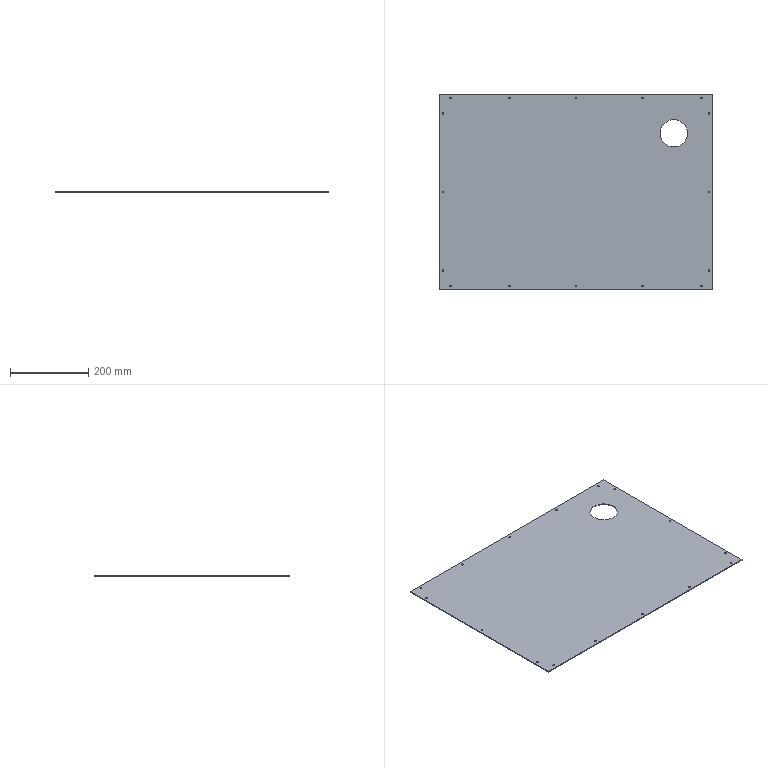Part | SolidWorks | features Extrusion 1, HoleWzd 1, ICE 1 | 1 solid | 40 faces | box 700 x 500 x 2 mm | volume 691794 mm3 | cylinder 34 | plane 6 | commonest cylinder face diameters 4.5 x32 70 x2
STEP:
#1=CARTESIAN_POINT('',(215.,150.,0.));
#2=VERTEX_POINT('',#1);
#3=CARTESIAN_POINT('',(285.,150.,0.));
#4=VERTEX_POINT('',#3);
#5=CARTESIAN_POINT('',(250.,150.,0.));
#6=DIRECTION('',(0.,0.,1.));
#7=DIRECTION('',(1.,0.,0.));
#8=AXIS2_PLACEMENT_3D('',#5,#6,#7);
#9=CIRCLE('',#8,35.);
#10=EDGE_CURVE('',#2,#4,#9,.T.);
#11=ORIENTED_EDGE('',*,*,#10,.F.);
#12=CARTESIAN_POINT('',(215.,150.,2.));
#13=VERTEX_POINT('',#12);
#14=CARTESIAN_POINT('',(215.,150.,-8.));
#15=DIRECTION('',(0.,0.,1.));
#16=VECTOR('',#15,1000.);
#17=LINE('',#14,#16);
#18=EDGE_CURVE('',#2,#13,#17,.T.);
#19=ORIENTED_EDGE('',*,*,#18,.T.);
#20=CARTESIAN_POINT('',(285.,150.,2.));
#21=VERTEX_POINT('',#20);
#22=CARTESIAN_POINT('',(250.,150.,2.));
#23=DIRECTION('',(0.,0.,1.));
#24=DIRECTION('',(1.,0.,0.));
#25=AXIS2_PLACEMENT_3D('',#22,#23,#24);
#26=CIRCLE('',#25,35.);
#27=EDGE_CURVE('',#13,#21,#26,.T.);
#28=ORIENTED_EDGE('',*,*,#27,.T.);
#29=CARTESIAN_POINT('',(285.,150.,-8.));
#30=DIRECTION('',(0.,0.,1.));
#31=VECTOR('',#30,1000.);
#32=LINE('',#29,#31);
#33=EDGE_CURVE('',#4,#21,#32,.T.);
#34=ORIENTED_EDGE('',*,*,#33,.F.);
#35=EDGE_LOOP('',(#11,#19,#28,#34));
#36=FACE_OUTER_BOUND('',#35,.T.);
#37=CARTESIAN_POINT('',(250.,150.,-8.));
#38=DIRECTION('',(0.,0.,1.));
#39=DIRECTION('',(1.,0.,0.));
#40=AXIS2_PLACEMENT_3D('',#37,#38,#39);
#41=CYLINDRICAL_SURFACE('',#40,35.);
#42=ADVANCED_FACE('',(#36),#41,.F.);
#43=CARTESIAN_POINT('',(-342.25,0.,0.));
#44=VERTEX_POINT('',#43);
#45=CARTESIAN_POINT('',(-337.75,0.,0.));
#46=VERTEX_POINT('',#45);
#47=CARTESIAN_POINT('',(-340.,0.,0.));
#48=DIRECTION('',(0.,0.,1.));
#49=DIRECTION('',(1.,0.,0.));
#50=AXIS2_PLACEMENT_3D('',#47,#48,#49);
#51=CIRCLE('',#50,2.25);
#52=EDGE_CURVE('',#44,#46,#51,.T.);
#53=ORIENTED_EDGE('',*,*,#52,.F.);
#54=CARTESIAN_POINT('',(-342.25,0.,2.));
#55=VERTEX_POINT('',#54);
#56=CARTESIAN_POINT('',(-342.25,0.,2.));
#57=DIRECTION('',(0.,0.,1.));
#58=VECTOR('',#57,1000.);
#59=LINE('',#56,#58);
#60=EDGE_CURVE('',#44,#55,#59,.T.);
#61=ORIENTED_EDGE('',*,*,#60,.T.);
#62=CARTESIAN_POINT('',(-337.75,0.,2.));
#63=VERTEX_POINT('',#62);
#64=CARTESIAN_POINT('',(-340.,0.,2.));
#65=DIRECTION('',(0.,0.,1.));
#66=DIRECTION('',(1.,0.,0.));
#67=AXIS2_PLACEMENT_3D('',#64,#65,#66);
#68=CIRCLE('',#67,2.25);
#69=EDGE_CURVE('',#55,#63,#68,.T.);
#70=ORIENTED_EDGE('',*,*,#69,.T.);
#71=CARTESIAN_POINT('',(-337.75,0.,2.));
#72=DIRECTION('',(0.,0.,1.));
#73=VECTOR('',#72,1000.);
#74=LINE('',#71,#73);
#75=EDGE_CURVE('',#46,#63,#74,.T.);
#76=ORIENTED_EDGE('',*,*,#75,.F.);
#77=EDGE_LOOP('',(#53,#61,#70,#76));
#78=FACE_OUTER_BOUND('',#77,.T.);
#79=CARTESIAN_POINT('',(-340.,0.,2.));
#80=DIRECTION('',(0.,0.,1.));
#81=DIRECTION('',(1.,0.,0.));
#82=AXIS2_PLACEMENT_3D('',#79,#80,#81);
#83=CYLINDRICAL_SURFACE('',#82,2.25);
#84=ADVANCED_FACE('',(#78),#83,.F.);
#85=CARTESIAN_POINT('',(-2.25,-240.,0.));
#86=VERTEX_POINT('',#85);
#87=CARTESIAN_POINT('',(2.25,-240.,0.));
#88=VERTEX_POINT('',#87);
#89=CARTESIAN_POINT('',(0.,-240.,0.));
#90=DIRECTION('',(0.,0.,1.));
#91=DIRECTION('',(1.,0.,0.));
#92=AXIS2_PLACEMENT_3D('',#89,#90,#91);
#93=CIRCLE('',#92,2.25);
#94=EDGE_CURVE('',#86,#88,#93,.T.);
#95=ORIENTED_EDGE('',*,*,#94,.F.);
#96=CARTESIAN_POINT('',(-2.25,-240.,2.));
#97=VERTEX_POINT('',#96);
#98=CARTESIAN_POINT('',(-2.25,-240.,2.));
#99=DIRECTION('',(0.,0.,1.));
#100=VECTOR('',#99,1000.);
#101=LINE('',#98,#100);
#102=EDGE_CURVE('',#86,#97,#101,.T.);
#103=ORIENTED_EDGE('',*,*,#102,.T.);
#104=CARTESIAN_POINT('',(2.25,-240.,2.));
#105=VERTEX_POINT('',#104);
#106=CARTESIAN_POINT('',(0.,-240.,2.));
#107=DIRECTION('',(0.,0.,1.));
#108=DIRECTION('',(1.,0.,0.));
#109=AXIS2_PLACEMENT_3D('',#106,#107,#108);
#110=CIRCLE('',#109,2.25);
#111=EDGE_CURVE('',#97,#105,#110,.T.);
#112=ORIENTED_EDGE('',*,*,#111,.T.);
#113=CARTESIAN_POINT('',(2.25,-240.,2.));
#114=DIRECTION('',(0.,0.,1.));
#115=VECTOR('',#114,1000.);
#116=LINE('',#113,#115);
#117=EDGE_CURVE('',#88,#105,#116,.T.);
#118=ORIENTED_EDGE('',*,*,#117,.F.);
#119=EDGE_LOOP('',(#95,#103,#112,#118));
#120=FACE_OUTER_BOUND('',#119,.T.);
#121=CARTESIAN_POINT('',(0.,-240.,2.));
#122=DIRECTION('',(0.,0.,1.));
#123=DIRECTION('',(1.,0.,0.));
#124=AXIS2_PLACEMENT_3D('',#121,#122,#123);
#125=CYLINDRICAL_SURFACE('',#124,2.25);
#126=ADVANCED_FACE('',(#120),#125,.F.);
#127=CARTESIAN_POINT('',(337.75,0.,0.));
#128=VERTEX_POINT('',#127);
#129=CARTESIAN_POINT('',(342.25,0.,0.));
#130=VERTEX_POINT('',#129);
#131=CARTESIAN_POINT('',(340.,0.,0.));
#132=DIRECTION('',(0.,0.,1.));
#133=DIRECTION('',(1.,0.,0.));
#134=AXIS2_PLACEMENT_3D('',#131,#132,#133);
#135=CIRCLE('',#134,2.25);
#136=EDGE_CURVE('',#128,#130,#135,.T.);
#137=ORIENTED_EDGE('',*,*,#136,.F.);
#138=CARTESIAN_POINT('',(337.75,0.,2.));
#139=VERTEX_POINT('',#138);
#140=CARTESIAN_POINT('',(337.75,0.,2.));
#141=DIRECTION('',(0.,0.,1.));
#142=VECTOR('',#141,1000.);
#143=LINE('',#140,#142);
#144=EDGE_CURVE('',#128,#139,#143,.T.);
#145=ORIENTED_EDGE('',*,*,#144,.T.);
#146=CARTESIAN_POINT('',(342.25,0.,2.));
#147=VERTEX_POINT('',#146);
#148=CARTESIAN_POINT('',(340.,0.,2.));
#149=DIRECTION('',(0.,0.,1.));
#150=DIRECTION('',(1.,0.,0.));
#151=AXIS2_PLACEMENT_3D('',#148,#149,#150);
#152=CIRCLE('',#151,2.25);
#153=EDGE_CURVE('',#139,#147,#152,.T.);
#154=ORIENTED_EDGE('',*,*,#153,.T.);
#155=CARTESIAN_POINT('',(342.25,0.,2.));
#156=DIRECTION('',(0.,0.,1.));
#157=VECTOR('',#156,1000.);
#158=LINE('',#155,#157);
#159=EDGE_CURVE('',#130,#147,#158,.T.);
#160=ORIENTED_EDGE('',*,*,#159,.F.);
#161=EDGE_LOOP('',(#137,#145,#154,#160));
#162=FACE_OUTER_BOUND('',#161,.T.);
#163=CARTESIAN_POINT('',(340.,0.,2.));
#164=DIRECTION('',(0.,0.,1.));
#165=DIRECTION('',(1.,0.,0.));
#166=AXIS2_PLACEMENT_3D('',#163,#164,#165);
#167=CYLINDRICAL_SURFACE('',#166,2.25);
#168=ADVANCED_FACE('',(#162),#167,.F.);
#169=CARTESIAN_POINT('',(-2.25,240.,0.));
#170=VERTEX_POINT('',#169);
#171=CARTESIAN_POINT('',(2.25,240.,0.));
#172=VERTEX_POINT('',#171);
#173=CARTESIAN_POINT('',(0.,240.,0.));
#174=DIRECTION('',(0.,0.,1.));
#175=DIRECTION('',(1.,0.,0.));
#176=AXIS2_PLACEMENT_3D('',#173,#174,#175);
#177=CIRCLE('',#176,2.25);
#178=EDGE_CURVE('',#170,#172,#177,.T.);
#179=ORIENTED_EDGE('',*,*,#178,.F.);
#180=CARTESIAN_POINT('',(-2.25,240.,2.));
#181=VERTEX_POINT('',#180);
#182=CARTESIAN_POINT('',(-2.25,240.,2.));
#183=DIRECTION('',(0.,0.,1.));
#184=VECTOR('',#183,1000.);
#185=LINE('',#182,#184);
#186=EDGE_CURVE('',#170,#181,#185,.T.);
#187=ORIENTED_EDGE('',*,*,#186,.T.);
#188=CARTESIAN_POINT('',(2.25,240.,2.));
#189=VERTEX_POINT('',#188);
#190=CARTESIAN_POINT('',(0.,240.,2.));
#191=DIRECTION('',(0.,0.,1.));
#192=DIRECTION('',(1.,0.,0.));
#193=AXIS2_PLACEMENT_3D('',#190,#191,#192);
#194=CIRCLE('',#193,2.25);
#195=EDGE_CURVE('',#181,#189,#194,.T.);
#196=ORIENTED_EDGE('',*,*,#195,.T.);
#197=CARTESIAN_POINT('',(2.25,240.,2.));
#198=DIRECTION('',(0.,0.,1.));
#199=VECTOR('',#198,1000.);
#200=LINE('',#197,#199);
#201=EDGE_CURVE('',#172,#189,#200,.T.);
#202=ORIENTED_EDGE('',*,*,#201,.F.);
#203=EDGE_LOOP('',(#179,#187,#196,#202));
#204=FACE_OUTER_BOUND('',#203,.T.);
#205=CARTESIAN_POINT('',(0.,240.,2.));
#206=DIRECTION('',(0.,0.,1.));
#207=DIRECTION('',(1.,0.,0.));
#208=AXIS2_PLACEMENT_3D('',#205,#206,#207);
#209=CYLINDRICAL_SURFACE('',#208,2.25);
#210=ADVANCED_FACE('',(#204),#209,.F.);
#211=CARTESIAN_POINT('',(-172.25,240.,0.));
#212=VERTEX_POINT('',#211);
#213=CARTESIAN_POINT('',(-167.75,240.,0.));
#214=VERTEX_POINT('',#213);
#215=CARTESIAN_POINT('',(-170.,240.,0.));
#216=DIRECTION('',(0.,0.,1.));
#217=DIRECTION('',(1.,0.,0.));
#218=AXIS2_PLACEMENT_3D('',#215,#216,#217);
#219=CIRCLE('',#218,2.25);
#220=EDGE_CURVE('',#212,#214,#219,.T.);
#221=ORIENTED_EDGE('',*,*,#220,.F.);
#222=CARTESIAN_POINT('',(-172.25,240.,2.));
#223=VERTEX_POINT('',#222);
#224=CARTESIAN_POINT('',(-172.25,240.,2.));
#225=DIRECTION('',(0.,0.,1.));
#226=VECTOR('',#225,1000.);
#227=LINE('',#224,#226);
#228=EDGE_CURVE('',#212,#223,#227,.T.);
#229=ORIENTED_EDGE('',*,*,#228,.T.);
#230=CARTESIAN_POINT('',(-167.75,240.,2.));
#231=VERTEX_POINT('',#230);
#232=CARTESIAN_POINT('',(-170.,240.,2.));
#233=DIRECTION('',(0.,0.,1.));
#234=DIRECTION('',(1.,0.,0.));
#235=AXIS2_PLACEMENT_3D('',#232,#233,#234);
#236=CIRCLE('',#235,2.25);
#237=EDGE_CURVE('',#223,#231,#236,.T.);
#238=ORIENTED_EDGE('',*,*,#237,.T.);
#239=CARTESIAN_POINT('',(-167.75,240.,2.));
#240=DIRECTION('',(0.,0.,1.));
#241=VECTOR('',#240,1000.);
#242=LINE('',#239,#241);
#243=EDGE_CURVE('',#214,#231,#242,.T.);
#244=ORIENTED_EDGE('',*,*,#243,.F.);
#245=EDGE_LOOP('',(#221,#229,#238,#244));
#246=FACE_OUTER_BOUND('',#245,.T.);
#247=CARTESIAN_POINT('',(-170.,240.,2.));
#248=DIRECTION('',(0.,0.,1.));
#249=DIRECTION('',(1.,0.,0.));
#250=AXIS2_PLACEMENT_3D('',#247,#248,#249);
#251=CYLINDRICAL_SURFACE('',#250,2.25);
#252=ADVANCED_FACE('',(#246),#251,.F.);
#253=CARTESIAN_POINT('',(167.75,240.,0.));
#254=VERTEX_POINT('',#253);
#255=CARTESIAN_POINT('',(172.25,240.,0.));
#256=VERTEX_POINT('',#255);
#257=CARTESIAN_POINT('',(170.,240.,0.));
#258=DIRECTION('',(0.,0.,1.));
#259=DIRECTION('',(1.,0.,0.));
#260=AXIS2_PLACEMENT_3D('',#257,#258,#259);
#261=CIRCLE('',#260,2.25);
#262=EDGE_CURVE('',#254,#256,#261,.T.);
#263=ORIENTED_EDGE('',*,*,#262,.F.);
#264=CARTESIAN_POINT('',(167.75,240.,2.));
#265=VERTEX_POINT('',#264);
#266=CARTESIAN_POINT('',(167.75,240.,2.));
#267=DIRECTION('',(0.,0.,1.));
#268=VECTOR('',#267,1000.);
#269=LINE('',#266,#268);
#270=EDGE_CURVE('',#254,#265,#269,.T.);
#271=ORIENTED_EDGE('',*,*,#270,.T.);
#272=CARTESIAN_POINT('',(172.25,240.,2.));
#273=VERTEX_POINT('',#272);
#274=CARTESIAN_POINT('',(170.,240.,2.));
#275=DIRECTION('',(0.,0.,1.));
#276=DIRECTION('',(1.,0.,0.));
#277=AXIS2_PLACEMENT_3D('',#274,#275,#276);
#278=CIRCLE('',#277,2.25);
#279=EDGE_CURVE('',#265,#273,#278,.T.);
#280=ORIENTED_EDGE('',*,*,#279,.T.);
#281=CARTESIAN_POINT('',(172.25,240.,2.));
#282=DIRECTION('',(0.,0.,1.));
#283=VECTOR('',#282,1000.);
#284=LINE('',#281,#283);
#285=EDGE_CURVE('',#256,#273,#284,.T.);
#286=ORIENTED_EDGE('',*,*,#285,.F.);
#287=EDGE_LOOP('',(#263,#271,#280,#286));
#288=FACE_OUTER_BOUND('',#287,.T.);
#289=CARTESIAN_POINT('',(170.,240.,2.));
#290=DIRECTION('',(0.,0.,1.));
#291=DIRECTION('',(1.,0.,0.));
#292=AXIS2_PLACEMENT_3D('',#289,#290,#291);
#293=CYLINDRICAL_SURFACE('',#292,2.25);
#294=ADVANCED_FACE('',(#288),#293,.F.);
#295=CARTESIAN_POINT('',(-172.25,-240.,0.));
#296=VERTEX_POINT('',#295);
#297=CARTESIAN_POINT('',(-167.75,-240.,0.));
#298=VERTEX_POINT('',#297);
#299=CARTESIAN_POINT('',(-170.,-240.,0.));
#300=DIRECTION('',(0.,0.,1.));
#301=DIRECTION('',(1.,0.,0.));
#302=AXIS2_PLACEMENT_3D('',#299,#300,#301);
#303=CIRCLE('',#302,2.25);
#304=EDGE_CURVE('',#296,#298,#303,.T.);
#305=ORIENTED_EDGE('',*,*,#304,.F.);
#306=CARTESIAN_POINT('',(-172.25,-240.,2.));
#307=VERTEX_POINT('',#306);
#308=CARTESIAN_POINT('',(-172.25,-240.,2.));
#309=DIRECTION('',(0.,0.,1.));
#310=VECTOR('',#309,1000.);
#311=LINE('',#308,#310);
#312=EDGE_CURVE('',#296,#307,#311,.T.);
#313=ORIENTED_EDGE('',*,*,#312,.T.);
#314=CARTESIAN_POINT('',(-167.75,-240.,2.));
#315=VERTEX_POINT('',#314);
#316=CARTESIAN_POINT('',(-170.,-240.,2.));
#317=DIRECTION('',(0.,0.,1.));
#318=DIRECTION('',(1.,0.,0.));
#319=AXIS2_PLACEMENT_3D('',#316,#317,#318);
#320=CIRCLE('',#319,2.25);
#321=EDGE_CURVE('',#307,#315,#320,.T.);
#322=ORIENTED_EDGE('',*,*,#321,.T.);
#323=CARTESIAN_POINT('',(-167.75,-240.,2.));
#324=DIRECTION('',(0.,0.,1.));
#325=VECTOR('',#324,1000.);
#326=LINE('',#323,#325);
#327=EDGE_CURVE('',#298,#315,#326,.T.);
#328=ORIENTED_EDGE('',*,*,#327,.F.);
#329=EDGE_LOOP('',(#305,#313,#322,#328));
#330=FACE_OUTER_BOUND('',#329,.T.);
#331=CARTESIAN_POINT('',(-170.,-240.,2.));
#332=DIRECTION('',(0.,0.,1.));
#333=DIRECTION('',(1.,0.,0.));
#334=AXIS2_PLACEMENT_3D('',#331,#332,#333);
#335=CYLINDRICAL_SURFACE('',#334,2.25);
#336=ADVANCED_FACE('',(#330),#335,.F.);
#337=CARTESIAN_POINT('',(167.75,-240.,0.));
#338=VERTEX_POINT('',#337);
#339=CARTESIAN_POINT('',(172.25,-240.,0.));
#340=VERTEX_POINT('',#339);
#341=CARTESIAN_POINT('',(170.,-240.,0.));
#342=DIRECTION('',(0.,0.,1.));
#343=DIRECTION('',(1.,0.,0.));
#344=AXIS2_PLACEMENT_3D('',#341,#342,#343);
#345=CIRCLE('',#344,2.25);
#346=EDGE_CURVE('',#338,#340,#345,.T.);
#347=ORIENTED_EDGE('',*,*,#346,.F.);
#348=CARTESIAN_POINT('',(167.75,-240.,2.));
#349=VERTEX_POINT('',#348);
#350=CARTESIAN_POINT('',(167.75,-240.,2.));
#351=DIRECTION('',(0.,0.,1.));
#352=VECTOR('',#351,1000.);
#353=LINE('',#350,#352);
#354=EDGE_CURVE('',#338,#349,#353,.T.);
#355=ORIENTED_EDGE('',*,*,#354,.T.);
#356=CARTESIAN_POINT('',(172.25,-240.,2.));
#357=VERTEX_POINT('',#356);
#358=CARTESIAN_POINT('',(170.,-240.,2.));
#359=DIRECTION('',(0.,0.,1.));
#360=DIRECTION('',(1.,0.,0.));
#361=AXIS2_PLACEMENT_3D('',#358,#359,#360);
#362=CIRCLE('',#361,2.25);
#363=EDGE_CURVE('',#349,#357,#362,.T.);
#364=ORIENTED_EDGE('',*,*,#363,.T.);
#365=CARTESIAN_POINT('',(172.25,-240.,2.));
#366=DIRECTION('',(0.,0.,1.));
#367=VECTOR('',#366,1000.);
#368=LINE('',#365,#367);
#369=EDGE_CURVE('',#340,#357,#368,.T.);
#370=ORIENTED_EDGE('',*,*,#369,.F.);
#371=EDGE_LOOP('',(#347,#355,#364,#370));
#372=FACE_OUTER_BOUND('',#371,.T.);
#373=CARTESIAN_POINT('',(170.,-240.,2.));
#374=DIRECTION('',(0.,0.,1.));
#375=DIRECTION('',(1.,0.,0.));
#376=AXIS2_PLACEMENT_3D('',#373,#374,#375);
#377=CYLINDRICAL_SURFACE('',#376,2.25);
#378=ADVANCED_FACE('',(#372),#377,.F.);
#379=CARTESIAN_POINT('',(-322.25,240.,0.));
#380=VERTEX_POINT('',#379);
#381=CARTESIAN_POINT('',(-317.75,240.,0.));
#382=VERTEX_POINT('',#381);
#383=CARTESIAN_POINT('',(-320.,240.,0.));
#384=DIRECTION('',(0.,0.,1.));
#385=DIRECTION('',(1.,0.,0.));
#386=AXIS2_PLACEMENT_3D('',#383,#384,#385);
#387=CIRCLE('',#386,2.25);
#388=EDGE_CURVE('',#380,#382,#387,.T.);
#389=ORIENTED_EDGE('',*,*,#388,.F.);
#390=CARTESIAN_POINT('',(-322.25,240.,2.));
#391=VERTEX_POINT('',#390);
#392=CARTESIAN_POINT('',(-322.25,240.,2.));
#393=DIRECTION('',(0.,0.,1.));
#394=VECTOR('',#393,1000.);
#395=LINE('',#392,#394);
#396=EDGE_CURVE('',#380,#391,#395,.T.);
#397=ORIENTED_EDGE('',*,*,#396,.T.);
#398=CARTESIAN_POINT('',(-317.75,240.,2.));
#399=VERTEX_POINT('',#398);
#400=CARTESIAN_POINT('',(-320.,240.,2.));
#401=DIRECTION('',(0.,0.,1.));
#402=DIRECTION('',(1.,0.,0.));
#403=AXIS2_PLACEMENT_3D('',#400,#401,#402);
#404=CIRCLE('',#403,2.25);
#405=EDGE_CURVE('',#391,#399,#404,.T.);
#406=ORIENTED_EDGE('',*,*,#405,.T.);
#407=CARTESIAN_POINT('',(-317.75,240.,2.));
#408=DIRECTION('',(0.,0.,1.));
#409=VECTOR('',#408,1000.);
#410=LINE('',#407,#409);
#411=EDGE_CURVE('',#382,#399,#410,.T.);
#412=ORIENTED_EDGE('',*,*,#411,.F.);
#413=EDGE_LOOP('',(#389,#397,#406,#412));
#414=FACE_OUTER_BOUND('',#413,.T.);
#415=CARTESIAN_POINT('',(-320.,240.,2.));
#416=DIRECTION('',(0.,0.,1.));
#417=DIRECTION('',(1.,0.,0.));
#418=AXIS2_PLACEMENT_3D('',#415,#416,#417);
#419=CYLINDRICAL_SURFACE('',#418,2.25);
#420=ADVANCED_FACE('',(#414),#419,.F.);
#421=CARTESIAN_POINT('',(317.75,240.,0.));
#422=VERTEX_POINT('',#421);
#423=CARTESIAN_POINT('',(322.25,240.,0.));
#424=VERTEX_POINT('',#423);
#425=CARTESIAN_POINT('',(320.,240.,0.));
#426=DIRECTION('',(0.,0.,1.));
#427=DIRECTION('',(1.,0.,0.));
#428=AXIS2_PLACEMENT_3D('',#425,#426,#427);
#429=CIRCLE('',#428,2.25);
#430=EDGE_CURVE('',#422,#424,#429,.T.);
#431=ORIENTED_EDGE('',*,*,#430,.F.);
#432=CARTESIAN_POINT('',(317.75,240.,2.));
#433=VERTEX_POINT('',#432);
#434=CARTESIAN_POINT('',(317.75,240.,2.));
#435=DIRECTION('',(0.,0.,1.));
#436=VECTOR('',#435,1000.);
#437=LINE('',#434,#436);
#438=EDGE_CURVE('',#422,#433,#437,.T.);
#439=ORIENTED_EDGE('',*,*,#438,.T.);
#440=CARTESIAN_POINT('',(322.25,240.,2.));
#441=VERTEX_POINT('',#440);
#442=CARTESIAN_POINT('',(320.,240.,2.));
#443=DIRECTION('',(0.,0.,1.));
#444=DIRECTION('',(1.,0.,0.));
#445=AXIS2_PLACEMENT_3D('',#442,#443,#444);
#446=CIRCLE('',#445,2.25);
#447=EDGE_CURVE('',#433,#441,#446,.T.);
#448=ORIENTED_EDGE('',*,*,#447,.T.);
#449=CARTESIAN_POINT('',(322.25,240.,2.));
#450=DIRECTION('',(0.,0.,1.));
#451=VECTOR('',#450,1000.);
#452=LINE('',#449,#451);
#453=EDGE_CURVE('',#424,#441,#452,.T.);
#454=ORIENTED_EDGE('',*,*,#453,.F.);
#455=EDGE_LOOP('',(#431,#439,#448,#454));
#456=FACE_OUTER_BOUND('',#455,.T.);
#457=CARTESIAN_POINT('',(320.,240.,2.));
#458=DIRECTION('',(0.,0.,1.));
#459=DIRECTION('',(1.,0.,0.));
#460=AXIS2_PLACEMENT_3D('',#457,#458,#459);
#461=CYLINDRICAL_SURFACE('',#460,2.25);
#462=ADVANCED_FACE('',(#456),#461,.F.);
#463=CARTESIAN_POINT('',(-342.25,200.,0.));
#464=VERTEX_POINT('',#463);
#465=CARTESIAN_POINT('',(-337.75,200.,0.));
#466=VERTEX_POINT('',#465);
#467=CARTESIAN_POINT('',(-340.,200.,0.));
#468=DIRECTION('',(0.,0.,1.));
#469=DIRECTION('',(1.,0.,0.));
#470=AXIS2_PLACEMENT_3D('',#467,#468,#469);
#471=CIRCLE('',#470,2.25);
#472=EDGE_CURVE('',#464,#466,#471,.T.);
#473=ORIENTED_EDGE('',*,*,#472,.F.);
#474=CARTESIAN_POINT('',(-342.25,200.,2.));
#475=VERTEX_POINT('',#474);
#476=CARTESIAN_POINT('',(-342.25,200.,2.));
#477=DIRECTION('',(0.,0.,1.));
#478=VECTOR('',#477,1000.);
#479=LINE('',#476,#478);
#480=EDGE_CURVE('',#464,#475,#479,.T.);
#481=ORIENTED_EDGE('',*,*,#480,.T.);
#482=CARTESIAN_POINT('',(-337.75,200.,2.));
#483=VERTEX_POINT('',#482);
#484=CARTESIAN_POINT('',(-340.,200.,2.));
#485=DIRECTION('',(0.,0.,1.));
#486=DIRECTION('',(1.,0.,0.));
#487=AXIS2_PLACEMENT_3D('',#484,#485,#486);
#488=CIRCLE('',#487,2.25);
#489=EDGE_CURVE('',#475,#483,#488,.T.);
#490=ORIENTED_EDGE('',*,*,#489,.T.);
#491=CARTESIAN_POINT('',(-337.75,200.,2.));
#492=DIRECTION('',(0.,0.,1.));
#493=VECTOR('',#492,1000.);
#494=LINE('',#491,#493);
#495=EDGE_CURVE('',#466,#483,#494,.T.);
#496=ORIENTED_EDGE('',*,*,#495,.F.);
#497=EDGE_LOOP('',(#473,#481,#490,#496));
#498=FACE_OUTER_BOUND('',#497,.T.);
#499=CARTESIAN_POINT('',(-340.,200.,2.));
#500=DIRECTION('',(0.,0.,1.));
#501=DIRECTION('',(1.,0.,0.));
#502=AXIS2_PLACEMENT_3D('',#499,#500,#501);
#503=CYLINDRICAL_SURFACE('',#502,2.25);
#504=ADVANCED_FACE('',(#498),#503,.F.);
#505=CARTESIAN_POINT('',(-342.25,-200.,0.));
#506=VERTEX_POINT('',#505);
#507=CARTESIAN_POINT('',(-337.75,-200.,0.));
#508=VERTEX_POINT('',#507);
#509=CARTESIAN_POINT('',(-340.,-200.,0.));
#510=DIRECTION('',(0.,0.,1.));
#511=DIRECTION('',(1.,0.,0.));
#512=AXIS2_PLACEMENT_3D('',#509,#510,#511);
#513=CIRCLE('',#512,2.25);
#514=EDGE_CURVE('',#506,#508,#513,.T.);
#515=ORIENTED_EDGE('',*,*,#514,.F.);
#516=CARTESIAN_POINT('',(-342.25,-200.,2.));
#517=VERTEX_POINT('',#516);
#518=CARTESIAN_POINT('',(-342.25,-200.,2.));
#519=DIRECTION('',(0.,0.,1.));
#520=VECTOR('',#519,1000.);
#521=LINE('',#518,#520);
#522=EDGE_CURVE('',#506,#517,#521,.T.);
#523=ORIENTED_EDGE('',*,*,#522,.T.);
#524=CARTESIAN_POINT('',(-337.75,-200.,2.));
#525=VERTEX_POINT('',#524);
#526=CARTESIAN_POINT('',(-340.,-200.,2.));
#527=DIRECTION('',(0.,0.,1.));
#528=DIRECTION('',(1.,0.,0.));
#529=AXIS2_PLACEMENT_3D('',#526,#527,#528);
#530=CIRCLE('',#529,2.25);
#531=EDGE_CURVE('',#517,#525,#530,.T.);
#532=ORIENTED_EDGE('',*,*,#531,.T.);
#533=CARTESIAN_POINT('',(-337.75,-200.,2.));
#534=DIRECTION('',(0.,0.,1.));
#535=VECTOR('',#534,1000.);
#536=LINE('',#533,#535);
#537=EDGE_CURVE('',#508,#525,#536,.T.);
#538=ORIENTED_EDGE('',*,*,#537,.F.);
#539=EDGE_LOOP('',(#515,#523,#532,#538));
#540=FACE_OUTER_BOUND('',#539,.T.);
#541=CARTESIAN_POINT('',(-340.,-200.,2.));
#542=DIRECTION('',(0.,0.,1.));
#543=DIRECTION('',(1.,0.,0.));
#544=AXIS2_PLACEMENT_3D('',#541,#542,#543);
#545=CYLINDRICAL_SURFACE('',#544,2.25);
#546=ADVANCED_FACE('',(#540),#545,.F.);
#547=CARTESIAN_POINT('',(337.75,-200.,0.));
#548=VERTEX_POINT('',#547);
#549=CARTESIAN_POINT('',(342.25,-200.,0.));
#550=VERTEX_POINT('',#549);
#551=CARTESIAN_POINT('',(340.,-200.,0.));
#552=DIRECTION('',(0.,0.,1.));
#553=DIRECTION('',(1.,0.,0.));
#554=AXIS2_PLACEMENT_3D('',#551,#552,#553);
#555=CIRCLE('',#554,2.25);
#556=EDGE_CURVE('',#548,#550,#555,.T.);
#557=ORIENTED_EDGE('',*,*,#556,.F.);
#558=CARTESIAN_POINT('',(337.75,-200.,2.));
#559=VERTEX_POINT('',#558);
#560=CARTESIAN_POINT('',(337.75,-200.,2.));
#561=DIRECTION('',(0.,0.,1.));
#562=VECTOR('',#561,1000.);
#563=LINE('',#560,#562);
#564=EDGE_CURVE('',#548,#559,#563,.T.);
#565=ORIENTED_EDGE('',*,*,#564,.T.);
#566=CARTESIAN_POINT('',(342.25,-200.,2.));
#567=VERTEX_POINT('',#566);
#568=CARTESIAN_POINT('',(340.,-200.,2.));
#569=DIRECTION('',(0.,0.,1.));
#570=DIRECTION('',(1.,0.,0.));
#571=AXIS2_PLACEMENT_3D('',#568,#569,#570);
#572=CIRCLE('',#571,2.25);
#573=EDGE_CURVE('',#559,#567,#572,.T.);
#574=ORIENTED_EDGE('',*,*,#573,.T.);
#575=CARTESIAN_POINT('',(342.25,-200.,2.));
#576=DIRECTION('',(0.,0.,1.));
#577=VECTOR('',#576,1000.);
#578=LINE('',#575,#577);
#579=EDGE_CURVE('',#550,#567,#578,.T.);
#580=ORIENTED_EDGE('',*,*,#579,.F.);
#581=EDGE_LOOP('',(#557,#565,#574,#580));
#582=FACE_OUTER_BOUND('',#581,.T.);
#583=CARTESIAN_POINT('',(340.,-200.,2.));
#584=DIRECTION('',(0.,0.,1.));
#585=DIRECTION('',(1.,0.,0.));
#586=AXIS2_PLACEMENT_3D('',#583,#584,#585);
#587=CYLINDRICAL_SURFACE('',#586,2.25);
#588=ADVANCED_FACE('',(#582),#587,.F.);
#589=CARTESIAN_POINT('',(337.75,200.,0.));
#590=VERTEX_POINT('',#589);
#591=CARTESIAN_POINT('',(342.25,200.,0.));
#592=VERTEX_POINT('',#591);
#593=CARTESIAN_POINT('',(340.,200.,0.));
#594=DIRECTION('',(0.,0.,1.));
#595=DIRECTION('',(1.,0.,0.));
#596=AXIS2_PLACEMENT_3D('',#593,#594,#595);
#597=CIRCLE('',#596,2.25);
#598=EDGE_CURVE('',#590,#592,#597,.T.);
#599=ORIENTED_EDGE('',*,*,#598,.F.);
#600=CARTESIAN_POINT('',(337.75,200.,2.));
#601=VERTEX_POINT('',#600);
#602=CARTESIAN_POINT('',(337.75,200.,2.));
#603=DIRECTION('',(0.,0.,1.));
#604=VECTOR('',#603,1000.);
#605=LINE('',#602,#604);
#606=EDGE_CURVE('',#590,#601,#605,.T.);
#607=ORIENTED_EDGE('',*,*,#606,.T.);
#608=CARTESIAN_POINT('',(342.25,200.,2.));
#609=VERTEX_POINT('',#608);
#610=CARTESIAN_POINT('',(340.,200.,2.));
#611=DIRECTION('',(0.,0.,1.));
#612=DIRECTION('',(1.,0.,0.));
#613=AXIS2_PLACEMENT_3D('',#610,#611,#612);
#614=CIRCLE('',#613,2.25);
#615=EDGE_CURVE('',#601,#609,#614,.T.);
#616=ORIENTED_EDGE('',*,*,#615,.T.);
#617=CARTESIAN_POINT('',(342.25,200.,2.));
#618=DIRECTION('',(0.,0.,1.));
#619=VECTOR('',#618,1000.);
#620=LINE('',#617,#619);
#621=EDGE_CURVE('',#592,#609,#620,.T.);
#622=ORIENTED_EDGE('',*,*,#621,.F.);
#623=EDGE_LOOP('',(#599,#607,#616,#622));
#624=FACE_OUTER_BOUND('',#623,.T.);
#625=CARTESIAN_POINT('',(340.,200.,2.));
#626=DIRECTION('',(0.,0.,1.));
#627=DIRECTION('',(1.,0.,0.));
#628=AXIS2_PLACEMENT_3D('',#625,#626,#627);
#629=CYLINDRICAL_SURFACE('',#628,2.25);
#630=ADVANCED_FACE('',(#624),#629,.F.);
#631=CARTESIAN_POINT('',(-322.25,-240.,0.));
#632=VERTEX_POINT('',#631);
#633=CARTESIAN_POINT('',(-317.75,-240.,0.));
#634=VERTEX_POINT('',#633);
#635=CARTESIAN_POINT('',(-320.,-240.,0.));
#636=DIRECTION('',(0.,0.,1.));
#637=DIRECTION('',(1.,0.,0.));
#638=AXIS2_PLACEMENT_3D('',#635,#636,#637);
#639=CIRCLE('',#638,2.25);
#640=EDGE_CURVE('',#632,#634,#639,.T.);
#641=ORIENTED_EDGE('',*,*,#640,.F.);
#642=CARTESIAN_POINT('',(-322.25,-240.,2.));
#643=VERTEX_POINT('',#642);
#644=CARTESIAN_POINT('',(-322.25,-240.,2.));
#645=DIRECTION('',(0.,0.,1.));
#646=VECTOR('',#645,1000.);
#647=LINE('',#644,#646);
#648=EDGE_CURVE('',#632,#643,#647,.T.);
#649=ORIENTED_EDGE('',*,*,#648,.T.);
#650=CARTESIAN_POINT('',(-317.75,-240.,2.));
#651=VERTEX_POINT('',#650);
#652=CARTESIAN_POINT('',(-320.,-240.,2.));
#653=DIRECTION('',(0.,0.,1.));
#654=DIRECTION('',(1.,0.,0.));
#655=AXIS2_PLACEMENT_3D('',#652,#653,#654);
#656=CIRCLE('',#655,2.25);
#657=EDGE_CURVE('',#643,#651,#656,.T.);
#658=ORIENTED_EDGE('',*,*,#657,.T.);
#659=CARTESIAN_POINT('',(-317.75,-240.,2.));
#660=DIRECTION('',(0.,0.,1.));
#661=VECTOR('',#660,1000.);
#662=LINE('',#659,#661);
#663=EDGE_CURVE('',#634,#651,#662,.T.);
#664=ORIENTED_EDGE('',*,*,#663,.F.);
#665=EDGE_LOOP('',(#641,#649,#658,#664));
#666=FACE_OUTER_BOUND('',#665,.T.);
#667=CARTESIAN_POINT('',(-320.,-240.,2.));
#668=DIRECTION('',(0.,0.,1.));
#669=DIRECTION('',(1.,0.,0.));
#670=AXIS2_PLACEMENT_3D('',#667,#668,#669);
#671=CYLINDRICAL_SURFACE('',#670,2.25);
#672=ADVANCED_FACE('',(#666),#671,.F.);
#673=CARTESIAN_POINT('',(317.75,-240.,0.));
#674=VERTEX_POINT('',#673);
#675=CARTESIAN_POINT('',(322.25,-240.,0.));
#676=VERTEX_POINT('',#675);
#677=CARTESIAN_POINT('',(320.,-240.,0.));
#678=DIRECTION('',(0.,0.,1.));
#679=DIRECTION('',(1.,0.,0.));
#680=AXIS2_PLACEMENT_3D('',#677,#678,#679);
#681=CIRCLE('',#680,2.25);
#682=EDGE_CURVE('',#674,#676,#681,.T.);
#683=ORIENTED_EDGE('',*,*,#682,.F.);
#684=CARTESIAN_POINT('',(317.75,-240.,2.));
#685=VERTEX_POINT('',#684);
#686=CARTESIAN_POINT('',(317.75,-240.,2.));
#687=DIRECTION('',(0.,0.,1.));
#688=VECTOR('',#687,1000.);
#689=LINE('',#686,#688);
#690=EDGE_CURVE('',#674,#685,#689,.T.);
#691=ORIENTED_EDGE('',*,*,#690,.T.);
#692=CARTESIAN_POINT('',(322.25,-240.,2.));
#693=VERTEX_POINT('',#692);
#694=CARTESIAN_POINT('',(320.,-240.,2.));
#695=DIRECTION('',(0.,0.,1.));
#696=DIRECTION('',(1.,0.,0.));
#697=AXIS2_PLACEMENT_3D('',#694,#695,#696);
#698=CIRCLE('',#697,2.25);
#699=EDGE_CURVE('',#685,#693,#698,.T.);
#700=ORIENTED_EDGE('',*,*,#699,.T.);
#701=CARTESIAN_POINT('',(322.25,-240.,2.));
#702=DIRECTION('',(0.,0.,1.));
#703=VECTOR('',#702,1000.);
#704=LINE('',#701,#703);
#705=EDGE_CURVE('',#676,#693,#704,.T.);
#706=ORIENTED_EDGE('',*,*,#705,.F.);
#707=EDGE_LOOP('',(#683,#691,#700,#706));
#708=FACE_OUTER_BOUND('',#707,.T.);
#709=CARTESIAN_POINT('',(320.,-240.,2.));
#710=DIRECTION('',(0.,0.,1.));
#711=DIRECTION('',(1.,0.,0.));
#712=AXIS2_PLACEMENT_3D('',#709,#710,#711);
#713=CYLINDRICAL_SURFACE('',#712,2.25);
#714=ADVANCED_FACE('',(#708),#713,.F.);
#715=CARTESIAN_POINT('',(350.,-250.,0.));
#716=VERTEX_POINT('',#715);
#717=CARTESIAN_POINT('',(350.,250.,0.));
#718=VERTEX_POINT('',#717);
#719=CARTESIAN_POINT('',(350.,250.,0.));
#720=DIRECTION('',(0.,1.,0.));
#721=VECTOR('',#720,1000.);
#722=LINE('',#719,#721);
#723=EDGE_CURVE('',#716,#718,#722,.T.);
#724=ORIENTED_EDGE('',*,*,#723,.T.);
#725=CARTESIAN_POINT('',(350.,250.,2.));
#726=VERTEX_POINT('',#725);
#727=CARTESIAN_POINT('',(350.,250.,2.));
#728=DIRECTION('',(0.,0.,-1.));
#729=VECTOR('',#728,1000.);
#730=LINE('',#727,#729);
#731=EDGE_CURVE('',#726,#718,#730,.T.);
#732=ORIENTED_EDGE('',*,*,#731,.F.);
#733=CARTESIAN_POINT('',(350.,-250.,2.));
#734=VERTEX_POINT('',#733);
#735=CARTESIAN_POINT('',(350.,250.,2.));
#736=DIRECTION('',(0.,1.,0.));
#737=VECTOR('',#736,1000.);
#738=LINE('',#735,#737);
#739=EDGE_CURVE('',#734,#726,#738,.T.);
#740=ORIENTED_EDGE('',*,*,#739,.F.);
#741=CARTESIAN_POINT('',(350.,-250.,2.));
#742=DIRECTION('',(0.,0.,-1.));
#743=VECTOR('',#742,1000.);
#744=LINE('',#741,#743);
#745=EDGE_CURVE('',#734,#716,#744,.T.);
#746=ORIENTED_EDGE('',*,*,#745,.T.);
#747=EDGE_LOOP('',(#724,#732,#740,#746));
#748=FACE_OUTER_BOUND('',#747,.T.);
#749=CARTESIAN_POINT('',(350.,250.,2.));
#750=DIRECTION('',(-1.,0.,0.));
#751=DIRECTION('',(0.,0.,1.));
#752=AXIS2_PLACEMENT_3D('',#749,#750,#751);
#753=PLANE('',#752);
#754=ADVANCED_FACE('',(#748),#753,.F.);
#755=CARTESIAN_POINT('',(-350.,250.,0.));
#756=VERTEX_POINT('',#755);
#757=CARTESIAN_POINT('',(-350.,250.,0.));
#758=DIRECTION('',(-1.,0.,0.));
#759=VECTOR('',#758,1000.);
#760=LINE('',#757,#759);
#761=EDGE_CURVE('',#718,#756,#760,.T.);
#762=ORIENTED_EDGE('',*,*,#761,.T.);
#763=CARTESIAN_POINT('',(-350.,250.,2.));
#764=VERTEX_POINT('',#763);
#765=CARTESIAN_POINT('',(-350.,250.,2.));
#766=DIRECTION('',(0.,0.,-1.));
#767=VECTOR('',#766,1000.);
#768=LINE('',#765,#767);
#769=EDGE_CURVE('',#764,#756,#768,.T.);
#770=ORIENTED_EDGE('',*,*,#769,.F.);
#771=CARTESIAN_POINT('',(-350.,250.,2.));
#772=DIRECTION('',(-1.,0.,0.));
#773=VECTOR('',#772,1000.);
#774=LINE('',#771,#773);
#775=EDGE_CURVE('',#726,#764,#774,.T.);
#776=ORIENTED_EDGE('',*,*,#775,.F.);
#777=ORIENTED_EDGE('',*,*,#731,.T.);
#778=EDGE_LOOP('',(#762,#770,#776,#777));
#779=FACE_OUTER_BOUND('',#778,.T.);
#780=CARTESIAN_POINT('',(-350.,250.,2.));
#781=DIRECTION('',(0.,-1.,0.));
#782=DIRECTION('',(0.,0.,-1.));
#783=AXIS2_PLACEMENT_3D('',#780,#781,#782);
#784=PLANE('',#783);
#785=ADVANCED_FACE('',(#779),#784,.F.);
#786=CARTESIAN_POINT('',(-350.,-250.,0.));
#787=VERTEX_POINT('',#786);
#788=CARTESIAN_POINT('',(-350.,250.,0.));
#789=DIRECTION('',(0.,-1.,0.));
#790=VECTOR('',#789,1000.);
#791=LINE('',#788,#790);
#792=EDGE_CURVE('',#756,#787,#791,.T.);
#793=ORIENTED_EDGE('',*,*,#792,.T.);
#794=CARTESIAN_POINT('',(-350.,-250.,2.));
#795=VERTEX_POINT('',#794);
#796=CARTESIAN_POINT('',(-350.,-250.,2.));
#797=DIRECTION('',(0.,0.,-1.));
#798=VECTOR('',#797,1000.);
#799=LINE('',#796,#798);
#800=EDGE_CURVE('',#795,#787,#799,.T.);
#801=ORIENTED_EDGE('',*,*,#800,.F.);
#802=CARTESIAN_POINT('',(-350.,250.,2.));
#803=DIRECTION('',(0.,-1.,0.));
#804=VECTOR('',#803,1000.);
#805=LINE('',#802,#804);
#806=EDGE_CURVE('',#764,#795,#805,.T.);
#807=ORIENTED_EDGE('',*,*,#806,.F.);
#808=ORIENTED_EDGE('',*,*,#769,.T.);
#809=EDGE_LOOP('',(#793,#801,#807,#808));
#810=FACE_OUTER_BOUND('',#809,.T.);
#811=CARTESIAN_POINT('',(-350.,250.,2.));
#812=DIRECTION('',(1.,0.,0.));
#813=DIRECTION('',(0.,0.,-1.));
#814=AXIS2_PLACEMENT_3D('',#811,#812,#813);
#815=PLANE('',#814);
#816=ADVANCED_FACE('',(#810),#815,.F.);
#817=CARTESIAN_POINT('',(-350.,-250.,0.));
#818=DIRECTION('',(1.,0.,0.));
#819=VECTOR('',#818,1000.);
#820=LINE('',#817,#819);
#821=EDGE_CURVE('',#787,#716,#820,.T.);
#822=ORIENTED_EDGE('',*,*,#821,.T.);
#823=ORIENTED_EDGE('',*,*,#745,.F.);
#824=CARTESIAN_POINT('',(-350.,-250.,2.));
#825=DIRECTION('',(1.,0.,0.));
#826=VECTOR('',#825,1000.);
#827=LINE('',#824,#826);
#828=EDGE_CURVE('',#795,#734,#827,.T.);
#829=ORIENTED_EDGE('',*,*,#828,.F.);
#830=ORIENTED_EDGE('',*,*,#800,.T.);
#831=EDGE_LOOP('',(#822,#823,#829,#830));
#832=FACE_OUTER_BOUND('',#831,.T.);
#833=CARTESIAN_POINT('',(-350.,-250.,2.));
#834=DIRECTION('',(0.,1.,0.));
#835=DIRECTION('',(0.,0.,1.));
#836=AXIS2_PLACEMENT_3D('',#833,#834,#835);
#837=PLANE('',#836);
#838=ADVANCED_FACE('',(#832),#837,.F.);
#839=CARTESIAN_POINT('',(250.,150.,2.));
#840=DIRECTION('',(0.,0.,1.));
#841=DIRECTION('',(1.,0.,0.));
#842=AXIS2_PLACEMENT_3D('',#839,#840,#841);
#843=CIRCLE('',#842,35.);
#844=EDGE_CURVE('',#21,#13,#843,.T.);
#845=ORIENTED_EDGE('',*,*,#844,.F.);
#846=ORIENTED_EDGE('',*,*,#27,.F.);
#847=EDGE_LOOP('',(#845,#846));
#848=FACE_BOUND('',#847,.T.);
#849=CARTESIAN_POINT('',(-340.,0.,2.));
#850=DIRECTION('',(0.,0.,1.));
#851=DIRECTION('',(1.,0.,0.));
#852=AXIS2_PLACEMENT_3D('',#849,#850,#851);
#853=CIRCLE('',#852,2.25);
#854=EDGE_CURVE('',#63,#55,#853,.T.);
#855=ORIENTED_EDGE('',*,*,#854,.F.);
#856=ORIENTED_EDGE('',*,*,#69,.F.);
#857=EDGE_LOOP('',(#855,#856));
#858=FACE_BOUND('',#857,.T.);
#859=CARTESIAN_POINT('',(0.,-240.,2.));
#860=DIRECTION('',(0.,0.,1.));
#861=DIRECTION('',(1.,0.,0.));
#862=AXIS2_PLACEMENT_3D('',#859,#860,#861);
#863=CIRCLE('',#862,2.25);
#864=EDGE_CURVE('',#105,#97,#863,.T.);
#865=ORIENTED_EDGE('',*,*,#864,.F.);
#866=ORIENTED_EDGE('',*,*,#111,.F.);
#867=EDGE_LOOP('',(#865,#866));
#868=FACE_BOUND('',#867,.T.);
#869=CARTESIAN_POINT('',(340.,0.,2.));
#870=DIRECTION('',(0.,0.,1.));
#871=DIRECTION('',(1.,0.,0.));
#872=AXIS2_PLACEMENT_3D('',#869,#870,#871);
#873=CIRCLE('',#872,2.25);
#874=EDGE_CURVE('',#147,#139,#873,.T.);
#875=ORIENTED_EDGE('',*,*,#874,.F.);
#876=ORIENTED_EDGE('',*,*,#153,.F.);
#877=EDGE_LOOP('',(#875,#876));
#878=FACE_BOUND('',#877,.T.);
#879=CARTESIAN_POINT('',(0.,240.,2.));
#880=DIRECTION('',(0.,0.,1.));
#881=DIRECTION('',(1.,0.,0.));
#882=AXIS2_PLACEMENT_3D('',#879,#880,#881);
#883=CIRCLE('',#882,2.25);
#884=EDGE_CURVE('',#189,#181,#883,.T.);
#885=ORIENTED_EDGE('',*,*,#884,.F.);
#886=ORIENTED_EDGE('',*,*,#195,.F.);
#887=EDGE_LOOP('',(#885,#886));
#888=FACE_BOUND('',#887,.T.);
#889=CARTESIAN_POINT('',(-170.,240.,2.));
#890=DIRECTION('',(0.,0.,1.));
#891=DIRECTION('',(1.,0.,0.));
#892=AXIS2_PLACEMENT_3D('',#889,#890,#891);
#893=CIRCLE('',#892,2.25);
#894=EDGE_CURVE('',#231,#223,#893,.T.);
#895=ORIENTED_EDGE('',*,*,#894,.F.);
#896=ORIENTED_EDGE('',*,*,#237,.F.);
#897=EDGE_LOOP('',(#895,#896));
#898=FACE_BOUND('',#897,.T.);
#899=CARTESIAN_POINT('',(170.,240.,2.));
#900=DIRECTION('',(0.,0.,1.));
#901=DIRECTION('',(1.,0.,0.));
#902=AXIS2_PLACEMENT_3D('',#899,#900,#901);
#903=CIRCLE('',#902,2.25);
#904=EDGE_CURVE('',#273,#265,#903,.T.);
#905=ORIENTED_EDGE('',*,*,#904,.F.);
#906=ORIENTED_EDGE('',*,*,#279,.F.);
#907=EDGE_LOOP('',(#905,#906));
#908=FACE_BOUND('',#907,.T.);
#909=CARTESIAN_POINT('',(-170.,-240.,2.));
#910=DIRECTION('',(0.,0.,1.));
#911=DIRECTION('',(1.,0.,0.));
#912=AXIS2_PLACEMENT_3D('',#909,#910,#911);
#913=CIRCLE('',#912,2.25);
#914=EDGE_CURVE('',#315,#307,#913,.T.);
#915=ORIENTED_EDGE('',*,*,#914,.F.);
#916=ORIENTED_EDGE('',*,*,#321,.F.);
#917=EDGE_LOOP('',(#915,#916));
#918=FACE_BOUND('',#917,.T.);
#919=CARTESIAN_POINT('',(170.,-240.,2.));
#920=DIRECTION('',(0.,0.,1.));
#921=DIRECTION('',(1.,0.,0.));
#922=AXIS2_PLACEMENT_3D('',#919,#920,#921);
#923=CIRCLE('',#922,2.25);
#924=EDGE_CURVE('',#357,#349,#923,.T.);
#925=ORIENTED_EDGE('',*,*,#924,.F.);
#926=ORIENTED_EDGE('',*,*,#363,.F.);
#927=EDGE_LOOP('',(#925,#926));
#928=FACE_BOUND('',#927,.T.);
#929=CARTESIAN_POINT('',(-320.,240.,2.));
#930=DIRECTION('',(0.,0.,1.));
#931=DIRECTION('',(1.,0.,0.));
#932=AXIS2_PLACEMENT_3D('',#929,#930,#931);
#933=CIRCLE('',#932,2.25);
#934=EDGE_CURVE('',#399,#391,#933,.T.);
#935=ORIENTED_EDGE('',*,*,#934,.F.);
#936=ORIENTED_EDGE('',*,*,#405,.F.);
#937=EDGE_LOOP('',(#935,#936));
#938=FACE_BOUND('',#937,.T.);
#939=CARTESIAN_POINT('',(320.,240.,2.));
#940=DIRECTION('',(0.,0.,1.));
#941=DIRECTION('',(1.,0.,0.));
#942=AXIS2_PLACEMENT_3D('',#939,#940,#941);
#943=CIRCLE('',#942,2.25);
#944=EDGE_CURVE('',#441,#433,#943,.T.);
#945=ORIENTED_EDGE('',*,*,#944,.F.);
#946=ORIENTED_EDGE('',*,*,#447,.F.);
#947=EDGE_LOOP('',(#945,#946));
#948=FACE_BOUND('',#947,.T.);
#949=CARTESIAN_POINT('',(-340.,200.,2.));
#950=DIRECTION('',(0.,0.,1.));
#951=DIRECTION('',(1.,0.,0.));
#952=AXIS2_PLACEMENT_3D('',#949,#950,#951);
#953=CIRCLE('',#952,2.25);
#954=EDGE_CURVE('',#483,#475,#953,.T.);
#955=ORIENTED_EDGE('',*,*,#954,.F.);
#956=ORIENTED_EDGE('',*,*,#489,.F.);
#957=EDGE_LOOP('',(#955,#956));
#958=FACE_BOUND('',#957,.T.);
#959=CARTESIAN_POINT('',(-340.,-200.,2.));
#960=DIRECTION('',(0.,0.,1.));
#961=DIRECTION('',(1.,0.,0.));
#962=AXIS2_PLACEMENT_3D('',#959,#960,#961);
#963=CIRCLE('',#962,2.25);
#964=EDGE_CURVE('',#525,#517,#963,.T.);
#965=ORIENTED_EDGE('',*,*,#964,.F.);
#966=ORIENTED_EDGE('',*,*,#531,.F.);
#967=EDGE_LOOP('',(#965,#966));
#968=FACE_BOUND('',#967,.T.);
#969=CARTESIAN_POINT('',(340.,-200.,2.));
#970=DIRECTION('',(0.,0.,1.));
#971=DIRECTION('',(1.,0.,0.));
#972=AXIS2_PLACEMENT_3D('',#969,#970,#971);
#973=CIRCLE('',#972,2.25);
#974=EDGE_CURVE('',#567,#559,#973,.T.);
#975=ORIENTED_EDGE('',*,*,#974,.F.);
#976=ORIENTED_EDGE('',*,*,#573,.F.);
#977=EDGE_LOOP('',(#975,#976));
#978=FACE_BOUND('',#977,.T.);
#979=CARTESIAN_POINT('',(340.,200.,2.));
#980=DIRECTION('',(0.,0.,1.));
#981=DIRECTION('',(1.,0.,0.));
#982=AXIS2_PLACEMENT_3D('',#979,#980,#981);
#983=CIRCLE('',#982,2.25);
#984=EDGE_CURVE('',#609,#601,#983,.T.);
#985=ORIENTED_EDGE('',*,*,#984,.F.);
#986=ORIENTED_EDGE('',*,*,#615,.F.);
#987=EDGE_LOOP('',(#985,#986));
#988=FACE_BOUND('',#987,.T.);
#989=CARTESIAN_POINT('',(-320.,-240.,2.));
#990=DIRECTION('',(0.,0.,1.));
#991=DIRECTION('',(1.,0.,0.));
#992=AXIS2_PLACEMENT_3D('',#989,#990,#991);
#993=CIRCLE('',#992,2.25);
#994=EDGE_CURVE('',#651,#643,#993,.T.);
#995=ORIENTED_EDGE('',*,*,#994,.F.);
#996=ORIENTED_EDGE('',*,*,#657,.F.);
#997=EDGE_LOOP('',(#995,#996));
#998=FACE_BOUND('',#997,.T.);
#999=CARTESIAN_POINT('',(320.,-240.,2.));
#1000=DIRECTION('',(0.,0.,1.));
#1001=DIRECTION('',(1.,0.,0.));
#1002=AXIS2_PLACEMENT_3D('',#999,#1000,#1001);
#1003=CIRCLE('',#1002,2.25);
#1004=EDGE_CURVE('',#693,#685,#1003,.T.);
#1005=ORIENTED_EDGE('',*,*,#1004,.F.);
#1006=ORIENTED_EDGE('',*,*,#699,.F.);
#1007=EDGE_LOOP('',(#1005,#1006));
#1008=FACE_BOUND('',#1007,.T.);
#1009=ORIENTED_EDGE('',*,*,#739,.T.);
#1010=ORIENTED_EDGE('',*,*,#775,.T.);
#1011=ORIENTED_EDGE('',*,*,#806,.T.);
#1012=ORIENTED_EDGE('',*,*,#828,.T.);
#1013=EDGE_LOOP('',(#1009,#1010,#1011,#1012));
#1014=FACE_OUTER_BOUND('',#1013,.T.);
#1015=CARTESIAN_POINT('',(0.,0.,2.));
#1016=DIRECTION('',(0.,0.,1.));
#1017=DIRECTION('',(1.,0.,0.));
#1018=AXIS2_PLACEMENT_3D('',#1015,#1016,#1017);
#1019=PLANE('',#1018);
#1020=ADVANCED_FACE('',(#848,#858,#868,#878,#888,#898,#908,#918,#928,#938,#948,#958,#968,#978,#988,#998,#1008,#1014),#1019,.T.);
#1021=CARTESIAN_POINT('',(250.,150.,0.));
#1022=DIRECTION('',(0.,0.,1.));
#1023=DIRECTION('',(1.,0.,0.));
#1024=AXIS2_PLACEMENT_3D('',#1021,#1022,#1023);
#1025=CIRCLE('',#1024,35.);
#1026=EDGE_CURVE('',#4,#2,#1025,.T.);
#1027=ORIENTED_EDGE('',*,*,#1026,.T.);
#1028=ORIENTED_EDGE('',*,*,#10,.T.);
#1029=EDGE_LOOP('',(#1027,#1028));
#1030=FACE_BOUND('',#1029,.T.);
#1031=CARTESIAN_POINT('',(-340.,0.,0.));
#1032=DIRECTION('',(0.,0.,1.));
#1033=DIRECTION('',(1.,0.,0.));
#1034=AXIS2_PLACEMENT_3D('',#1031,#1032,#1033);
#1035=CIRCLE('',#1034,2.25);
#1036=EDGE_CURVE('',#46,#44,#1035,.T.);
#1037=ORIENTED_EDGE('',*,*,#1036,.T.);
#1038=ORIENTED_EDGE('',*,*,#52,.T.);
#1039=EDGE_LOOP('',(#1037,#1038));
#1040=FACE_BOUND('',#1039,.T.);
#1041=CARTESIAN_POINT('',(0.,-240.,0.));
#1042=DIRECTION('',(0.,0.,1.));
#1043=DIRECTION('',(1.,0.,0.));
#1044=AXIS2_PLACEMENT_3D('',#1041,#1042,#1043);
#1045=CIRCLE('',#1044,2.25);
#1046=EDGE_CURVE('',#88,#86,#1045,.T.);
#1047=ORIENTED_EDGE('',*,*,#1046,.T.);
#1048=ORIENTED_EDGE('',*,*,#94,.T.);
#1049=EDGE_LOOP('',(#1047,#1048));
#1050=FACE_BOUND('',#1049,.T.);
#1051=CARTESIAN_POINT('',(340.,0.,0.));
#1052=DIRECTION('',(0.,0.,1.));
#1053=DIRECTION('',(1.,0.,0.));
#1054=AXIS2_PLACEMENT_3D('',#1051,#1052,#1053);
#1055=CIRCLE('',#1054,2.25);
#1056=EDGE_CURVE('',#130,#128,#1055,.T.);
#1057=ORIENTED_EDGE('',*,*,#1056,.T.);
#1058=ORIENTED_EDGE('',*,*,#136,.T.);
#1059=EDGE_LOOP('',(#1057,#1058));
#1060=FACE_BOUND('',#1059,.T.);
#1061=CARTESIAN_POINT('',(0.,240.,0.));
#1062=DIRECTION('',(0.,0.,1.));
#1063=DIRECTION('',(1.,0.,0.));
#1064=AXIS2_PLACEMENT_3D('',#1061,#1062,#1063);
#1065=CIRCLE('',#1064,2.25);
#1066=EDGE_CURVE('',#172,#170,#1065,.T.);
#1067=ORIENTED_EDGE('',*,*,#1066,.T.);
#1068=ORIENTED_EDGE('',*,*,#178,.T.);
#1069=EDGE_LOOP('',(#1067,#1068));
#1070=FACE_BOUND('',#1069,.T.);
#1071=CARTESIAN_POINT('',(-170.,240.,0.));
#1072=DIRECTION('',(0.,0.,1.));
#1073=DIRECTION('',(1.,0.,0.));
#1074=AXIS2_PLACEMENT_3D('',#1071,#1072,#1073);
#1075=CIRCLE('',#1074,2.25);
#1076=EDGE_CURVE('',#214,#212,#1075,.T.);
#1077=ORIENTED_EDGE('',*,*,#1076,.T.);
#1078=ORIENTED_EDGE('',*,*,#220,.T.);
#1079=EDGE_LOOP('',(#1077,#1078));
#1080=FACE_BOUND('',#1079,.T.);
#1081=CARTESIAN_POINT('',(170.,240.,0.));
#1082=DIRECTION('',(0.,0.,1.));
#1083=DIRECTION('',(1.,0.,0.));
#1084=AXIS2_PLACEMENT_3D('',#1081,#1082,#1083);
#1085=CIRCLE('',#1084,2.25);
#1086=EDGE_CURVE('',#256,#254,#1085,.T.);
#1087=ORIENTED_EDGE('',*,*,#1086,.T.);
#1088=ORIENTED_EDGE('',*,*,#262,.T.);
#1089=EDGE_LOOP('',(#1087,#1088));
#1090=FACE_BOUND('',#1089,.T.);
#1091=CARTESIAN_POINT('',(-170.,-240.,0.));
#1092=DIRECTION('',(0.,0.,1.));
#1093=DIRECTION('',(1.,0.,0.));
#1094=AXIS2_PLACEMENT_3D('',#1091,#1092,#1093);
#1095=CIRCLE('',#1094,2.25);
#1096=EDGE_CURVE('',#298,#296,#1095,.T.);
#1097=ORIENTED_EDGE('',*,*,#1096,.T.);
#1098=ORIENTED_EDGE('',*,*,#304,.T.);
#1099=EDGE_LOOP('',(#1097,#1098));
#1100=FACE_BOUND('',#1099,.T.);
#1101=CARTESIAN_POINT('',(170.,-240.,0.));
#1102=DIRECTION('',(0.,0.,1.));
#1103=DIRECTION('',(1.,0.,0.));
#1104=AXIS2_PLACEMENT_3D('',#1101,#1102,#1103);
#1105=CIRCLE('',#1104,2.25);
#1106=EDGE_CURVE('',#340,#338,#1105,.T.);
#1107=ORIENTED_EDGE('',*,*,#1106,.T.);
#1108=ORIENTED_EDGE('',*,*,#346,.T.);
#1109=EDGE_LOOP('',(#1107,#1108));
#1110=FACE_BOUND('',#1109,.T.);
#1111=CARTESIAN_POINT('',(-320.,240.,0.));
#1112=DIRECTION('',(0.,0.,1.));
#1113=DIRECTION('',(1.,0.,0.));
#1114=AXIS2_PLACEMENT_3D('',#1111,#1112,#1113);
#1115=CIRCLE('',#1114,2.25);
#1116=EDGE_CURVE('',#382,#380,#1115,.T.);
#1117=ORIENTED_EDGE('',*,*,#1116,.T.);
#1118=ORIENTED_EDGE('',*,*,#388,.T.);
#1119=EDGE_LOOP('',(#1117,#1118));
#1120=FACE_BOUND('',#1119,.T.);
#1121=CARTESIAN_POINT('',(320.,240.,0.));
#1122=DIRECTION('',(0.,0.,1.));
#1123=DIRECTION('',(1.,0.,0.));
#1124=AXIS2_PLACEMENT_3D('',#1121,#1122,#1123);
#1125=CIRCLE('',#1124,2.25);
#1126=EDGE_CURVE('',#424,#422,#1125,.T.);
#1127=ORIENTED_EDGE('',*,*,#1126,.T.);
#1128=ORIENTED_EDGE('',*,*,#430,.T.);
#1129=EDGE_LOOP('',(#1127,#1128));
#1130=FACE_BOUND('',#1129,.T.);
#1131=CARTESIAN_POINT('',(-340.,200.,0.));
#1132=DIRECTION('',(0.,0.,1.));
#1133=DIRECTION('',(1.,0.,0.));
#1134=AXIS2_PLACEMENT_3D('',#1131,#1132,#1133);
#1135=CIRCLE('',#1134,2.25);
#1136=EDGE_CURVE('',#466,#464,#1135,.T.);
#1137=ORIENTED_EDGE('',*,*,#1136,.T.);
#1138=ORIENTED_EDGE('',*,*,#472,.T.);
#1139=EDGE_LOOP('',(#1137,#1138));
#1140=FACE_BOUND('',#1139,.T.);
#1141=CARTESIAN_POINT('',(-340.,-200.,0.));
#1142=DIRECTION('',(0.,0.,1.));
#1143=DIRECTION('',(1.,0.,0.));
#1144=AXIS2_PLACEMENT_3D('',#1141,#1142,#1143);
#1145=CIRCLE('',#1144,2.25);
#1146=EDGE_CURVE('',#508,#506,#1145,.T.);
#1147=ORIENTED_EDGE('',*,*,#1146,.T.);
#1148=ORIENTED_EDGE('',*,*,#514,.T.);
#1149=EDGE_LOOP('',(#1147,#1148));
#1150=FACE_BOUND('',#1149,.T.);
#1151=CARTESIAN_POINT('',(340.,-200.,0.));
#1152=DIRECTION('',(0.,0.,1.));
#1153=DIRECTION('',(1.,0.,0.));
#1154=AXIS2_PLACEMENT_3D('',#1151,#1152,#1153);
#1155=CIRCLE('',#1154,2.25);
#1156=EDGE_CURVE('',#550,#548,#1155,.T.);
#1157=ORIENTED_EDGE('',*,*,#1156,.T.);
#1158=ORIENTED_EDGE('',*,*,#556,.T.);
#1159=EDGE_LOOP('',(#1157,#1158));
#1160=FACE_BOUND('',#1159,.T.);
#1161=CARTESIAN_POINT('',(340.,200.,0.));
#1162=DIRECTION('',(0.,0.,1.));
#1163=DIRECTION('',(1.,0.,0.));
#1164=AXIS2_PLACEMENT_3D('',#1161,#1162,#1163);
#1165=CIRCLE('',#1164,2.25);
#1166=EDGE_CURVE('',#592,#590,#1165,.T.);
#1167=ORIENTED_EDGE('',*,*,#1166,.T.);
#1168=ORIENTED_EDGE('',*,*,#598,.T.);
#1169=EDGE_LOOP('',(#1167,#1168));
#1170=FACE_BOUND('',#1169,.T.);
#1171=CARTESIAN_POINT('',(-320.,-240.,0.));
#1172=DIRECTION('',(0.,0.,1.));
#1173=DIRECTION('',(1.,0.,0.));
#1174=AXIS2_PLACEMENT_3D('',#1171,#1172,#1173);
#1175=CIRCLE('',#1174,2.25);
#1176=EDGE_CURVE('',#634,#632,#1175,.T.);
#1177=ORIENTED_EDGE('',*,*,#1176,.T.);
#1178=ORIENTED_EDGE('',*,*,#640,.T.);
#1179=EDGE_LOOP('',(#1177,#1178));
#1180=FACE_BOUND('',#1179,.T.);
#1181=CARTESIAN_POINT('',(320.,-240.,0.));
#1182=DIRECTION('',(0.,0.,1.));
#1183=DIRECTION('',(1.,0.,0.));
#1184=AXIS2_PLACEMENT_3D('',#1181,#1182,#1183);
#1185=CIRCLE('',#1184,2.25);
#1186=EDGE_CURVE('',#676,#674,#1185,.T.);
#1187=ORIENTED_EDGE('',*,*,#1186,.T.);
#1188=ORIENTED_EDGE('',*,*,#682,.T.);
#1189=EDGE_LOOP('',(#1187,#1188));
#1190=FACE_BOUND('',#1189,.T.);
#1191=ORIENTED_EDGE('',*,*,#723,.F.);
#1192=ORIENTED_EDGE('',*,*,#821,.F.);
#1193=ORIENTED_EDGE('',*,*,#792,.F.);
#1194=ORIENTED_EDGE('',*,*,#761,.F.);
#1195=EDGE_LOOP('',(#1191,#1192,#1193,#1194));
#1196=FACE_OUTER_BOUND('',#1195,.T.);
#1197=CARTESIAN_POINT('',(0.,0.,0.));
#1198=DIRECTION('',(0.,0.,1.));
#1199=DIRECTION('',(1.,0.,0.));
#1200=AXIS2_PLACEMENT_3D('',#1197,#1198,#1199);
#1201=PLANE('',#1200);
#1202=ADVANCED_FACE('',(#1030,#1040,#1050,#1060,#1070,#1080,#1090,#1100,#1110,#1120,#1130,#1140,#1150,#1160,#1170,#1180,#1190,#1196),#1201,.F.);
#1203=ORIENTED_EDGE('',*,*,#690,.F.);
#1204=ORIENTED_EDGE('',*,*,#1186,.F.);
#1205=ORIENTED_EDGE('',*,*,#705,.T.);
#1206=ORIENTED_EDGE('',*,*,#1004,.T.);
#1207=EDGE_LOOP('',(#1203,#1204,#1205,#1206));
#1208=FACE_OUTER_BOUND('',#1207,.T.);
#1209=CARTESIAN_POINT('',(320.,-240.,2.));
#1210=DIRECTION('',(0.,0.,1.));
#1211=DIRECTION('',(1.,0.,0.));
#1212=AXIS2_PLACEMENT_3D('',#1209,#1210,#1211);
#1213=CYLINDRICAL_SURFACE('',#1212,2.25);
#1214=ADVANCED_FACE('',(#1208),#1213,.F.);
#1215=ORIENTED_EDGE('',*,*,#648,.F.);
#1216=ORIENTED_EDGE('',*,*,#1176,.F.);
#1217=ORIENTED_EDGE('',*,*,#663,.T.);
#1218=ORIENTED_EDGE('',*,*,#994,.T.);
#1219=EDGE_LOOP('',(#1215,#1216,#1217,#1218));
#1220=FACE_OUTER_BOUND('',#1219,.T.);
#1221=CARTESIAN_POINT('',(-320.,-240.,2.));
#1222=DIRECTION('',(0.,0.,1.));
#1223=DIRECTION('',(1.,0.,0.));
#1224=AXIS2_PLACEMENT_3D('',#1221,#1222,#1223);
#1225=CYLINDRICAL_SURFACE('',#1224,2.25);
#1226=ADVANCED_FACE('',(#1220),#1225,.F.);
#1227=ORIENTED_EDGE('',*,*,#606,.F.);
#1228=ORIENTED_EDGE('',*,*,#1166,.F.);
#1229=ORIENTED_EDGE('',*,*,#621,.T.);
#1230=ORIENTED_EDGE('',*,*,#984,.T.);
#1231=EDGE_LOOP('',(#1227,#1228,#1229,#1230));
#1232=FACE_OUTER_BOUND('',#1231,.T.);
#1233=CARTESIAN_POINT('',(340.,200.,2.));
#1234=DIRECTION('',(0.,0.,1.));
#1235=DIRECTION('',(1.,0.,0.));
#1236=AXIS2_PLACEMENT_3D('',#1233,#1234,#1235);
#1237=CYLINDRICAL_SURFACE('',#1236,2.25);
#1238=ADVANCED_FACE('',(#1232),#1237,.F.);
#1239=ORIENTED_EDGE('',*,*,#564,.F.);
#1240=ORIENTED_EDGE('',*,*,#1156,.F.);
#1241=ORIENTED_EDGE('',*,*,#579,.T.);
#1242=ORIENTED_EDGE('',*,*,#974,.T.);
#1243=EDGE_LOOP('',(#1239,#1240,#1241,#1242));
#1244=FACE_OUTER_BOUND('',#1243,.T.);
#1245=CARTESIAN_POINT('',(340.,-200.,2.));
#1246=DIRECTION('',(0.,0.,1.));
#1247=DIRECTION('',(1.,0.,0.));
#1248=AXIS2_PLACEMENT_3D('',#1245,#1246,#1247);
#1249=CYLINDRICAL_SURFACE('',#1248,2.25);
#1250=ADVANCED_FACE('',(#1244),#1249,.F.);
#1251=ORIENTED_EDGE('',*,*,#522,.F.);
#1252=ORIENTED_EDGE('',*,*,#1146,.F.);
#1253=ORIENTED_EDGE('',*,*,#537,.T.);
#1254=ORIENTED_EDGE('',*,*,#964,.T.);
#1255=EDGE_LOOP('',(#1251,#1252,#1253,#1254));
#1256=FACE_OUTER_BOUND('',#1255,.T.);
#1257=CARTESIAN_POINT('',(-340.,-200.,2.));
#1258=DIRECTION('',(0.,0.,1.));
#1259=DIRECTION('',(1.,0.,0.));
#1260=AXIS2_PLACEMENT_3D('',#1257,#1258,#1259);
#1261=CYLINDRICAL_SURFACE('',#1260,2.25);
#1262=ADVANCED_FACE('',(#1256),#1261,.F.);
#1263=ORIENTED_EDGE('',*,*,#480,.F.);
#1264=ORIENTED_EDGE('',*,*,#1136,.F.);
#1265=ORIENTED_EDGE('',*,*,#495,.T.);
#1266=ORIENTED_EDGE('',*,*,#954,.T.);
#1267=EDGE_LOOP('',(#1263,#1264,#1265,#1266));
#1268=FACE_OUTER_BOUND('',#1267,.T.);
#1269=CARTESIAN_POINT('',(-340.,200.,2.));
#1270=DIRECTION('',(0.,0.,1.));
#1271=DIRECTION('',(1.,0.,0.));
#1272=AXIS2_PLACEMENT_3D('',#1269,#1270,#1271);
#1273=CYLINDRICAL_SURFACE('',#1272,2.25);
#1274=ADVANCED_FACE('',(#1268),#1273,.F.);
#1275=ORIENTED_EDGE('',*,*,#438,.F.);
#1276=ORIENTED_EDGE('',*,*,#1126,.F.);
#1277=ORIENTED_EDGE('',*,*,#453,.T.);
#1278=ORIENTED_EDGE('',*,*,#944,.T.);
#1279=EDGE_LOOP('',(#1275,#1276,#1277,#1278));
#1280=FACE_OUTER_BOUND('',#1279,.T.);
#1281=CARTESIAN_POINT('',(320.,240.,2.));
#1282=DIRECTION('',(0.,0.,1.));
#1283=DIRECTION('',(1.,0.,0.));
#1284=AXIS2_PLACEMENT_3D('',#1281,#1282,#1283);
#1285=CYLINDRICAL_SURFACE('',#1284,2.25);
#1286=ADVANCED_FACE('',(#1280),#1285,.F.);
#1287=ORIENTED_EDGE('',*,*,#396,.F.);
#1288=ORIENTED_EDGE('',*,*,#1116,.F.);
#1289=ORIENTED_EDGE('',*,*,#411,.T.);
#1290=ORIENTED_EDGE('',*,*,#934,.T.);
#1291=EDGE_LOOP('',(#1287,#1288,#1289,#1290));
#1292=FACE_OUTER_BOUND('',#1291,.T.);
#1293=CARTESIAN_POINT('',(-320.,240.,2.));
#1294=DIRECTION('',(0.,0.,1.));
#1295=DIRECTION('',(1.,0.,0.));
#1296=AXIS2_PLACEMENT_3D('',#1293,#1294,#1295);
#1297=CYLINDRICAL_SURFACE('',#1296,2.25);
#1298=ADVANCED_FACE('',(#1292),#1297,.F.);
#1299=ORIENTED_EDGE('',*,*,#354,.F.);
#1300=ORIENTED_EDGE('',*,*,#1106,.F.);
#1301=ORIENTED_EDGE('',*,*,#369,.T.);
#1302=ORIENTED_EDGE('',*,*,#924,.T.);
#1303=EDGE_LOOP('',(#1299,#1300,#1301,#1302));
#1304=FACE_OUTER_BOUND('',#1303,.T.);
#1305=CARTESIAN_POINT('',(170.,-240.,2.));
#1306=DIRECTION('',(0.,0.,1.));
#1307=DIRECTION('',(1.,0.,0.));
#1308=AXIS2_PLACEMENT_3D('',#1305,#1306,#1307);
#1309=CYLINDRICAL_SURFACE('',#1308,2.25);
#1310=ADVANCED_FACE('',(#1304),#1309,.F.);
#1311=ORIENTED_EDGE('',*,*,#312,.F.);
#1312=ORIENTED_EDGE('',*,*,#1096,.F.);
#1313=ORIENTED_EDGE('',*,*,#327,.T.);
#1314=ORIENTED_EDGE('',*,*,#914,.T.);
#1315=EDGE_LOOP('',(#1311,#1312,#1313,#1314));
#1316=FACE_OUTER_BOUND('',#1315,.T.);
#1317=CARTESIAN_POINT('',(-170.,-240.,2.));
#1318=DIRECTION('',(0.,0.,1.));
#1319=DIRECTION('',(1.,0.,0.));
#1320=AXIS2_PLACEMENT_3D('',#1317,#1318,#1319);
#1321=CYLINDRICAL_SURFACE('',#1320,2.25);
#1322=ADVANCED_FACE('',(#1316),#1321,.F.);
#1323=ORIENTED_EDGE('',*,*,#270,.F.);
#1324=ORIENTED_EDGE('',*,*,#1086,.F.);
#1325=ORIENTED_EDGE('',*,*,#285,.T.);
#1326=ORIENTED_EDGE('',*,*,#904,.T.);
#1327=EDGE_LOOP('',(#1323,#1324,#1325,#1326));
#1328=FACE_OUTER_BOUND('',#1327,.T.);
#1329=CARTESIAN_POINT('',(170.,240.,2.));
#1330=DIRECTION('',(0.,0.,1.));
#1331=DIRECTION('',(1.,0.,0.));
#1332=AXIS2_PLACEMENT_3D('',#1329,#1330,#1331);
#1333=CYLINDRICAL_SURFACE('',#1332,2.25);
#1334=ADVANCED_FACE('',(#1328),#1333,.F.);
#1335=ORIENTED_EDGE('',*,*,#228,.F.);
#1336=ORIENTED_EDGE('',*,*,#1076,.F.);
#1337=ORIENTED_EDGE('',*,*,#243,.T.);
#1338=ORIENTED_EDGE('',*,*,#894,.T.);
#1339=EDGE_LOOP('',(#1335,#1336,#1337,#1338));
#1340=FACE_OUTER_BOUND('',#1339,.T.);
#1341=CARTESIAN_POINT('',(-170.,240.,2.));
#1342=DIRECTION('',(0.,0.,1.));
#1343=DIRECTION('',(1.,0.,0.));
#1344=AXIS2_PLACEMENT_3D('',#1341,#1342,#1343);
#1345=CYLINDRICAL_SURFACE('',#1344,2.25);
#1346=ADVANCED_FACE('',(#1340),#1345,.F.);
#1347=ORIENTED_EDGE('',*,*,#186,.F.);
#1348=ORIENTED_EDGE('',*,*,#1066,.F.);
#1349=ORIENTED_EDGE('',*,*,#201,.T.);
#1350=ORIENTED_EDGE('',*,*,#884,.T.);
#1351=EDGE_LOOP('',(#1347,#1348,#1349,#1350));
#1352=FACE_OUTER_BOUND('',#1351,.T.);
#1353=CARTESIAN_POINT('',(0.,240.,2.));
#1354=DIRECTION('',(0.,0.,1.));
#1355=DIRECTION('',(1.,0.,0.));
#1356=AXIS2_PLACEMENT_3D('',#1353,#1354,#1355);
#1357=CYLINDRICAL_SURFACE('',#1356,2.25);
#1358=ADVANCED_FACE('',(#1352),#1357,.F.);
#1359=ORIENTED_EDGE('',*,*,#144,.F.);
#1360=ORIENTED_EDGE('',*,*,#1056,.F.);
#1361=ORIENTED_EDGE('',*,*,#159,.T.);
#1362=ORIENTED_EDGE('',*,*,#874,.T.);
#1363=EDGE_LOOP('',(#1359,#1360,#1361,#1362));
#1364=FACE_OUTER_BOUND('',#1363,.T.);
#1365=CARTESIAN_POINT('',(340.,0.,2.));
#1366=DIRECTION('',(0.,0.,1.));
#1367=DIRECTION('',(1.,0.,0.));
#1368=AXIS2_PLACEMENT_3D('',#1365,#1366,#1367);
#1369=CYLINDRICAL_SURFACE('',#1368,2.25);
#1370=ADVANCED_FACE('',(#1364),#1369,.F.);
#1371=ORIENTED_EDGE('',*,*,#102,.F.);
#1372=ORIENTED_EDGE('',*,*,#1046,.F.);
#1373=ORIENTED_EDGE('',*,*,#117,.T.);
#1374=ORIENTED_EDGE('',*,*,#864,.T.);
#1375=EDGE_LOOP('',(#1371,#1372,#1373,#1374));
#1376=FACE_OUTER_BOUND('',#1375,.T.);
#1377=CARTESIAN_POINT('',(0.,-240.,2.));
#1378=DIRECTION('',(0.,0.,1.));
#1379=DIRECTION('',(1.,0.,0.));
#1380=AXIS2_PLACEMENT_3D('',#1377,#1378,#1379);
#1381=CYLINDRICAL_SURFACE('',#1380,2.25);
#1382=ADVANCED_FACE('',(#1376),#1381,.F.);
#1383=ORIENTED_EDGE('',*,*,#60,.F.);
#1384=ORIENTED_EDGE('',*,*,#1036,.F.);
#1385=ORIENTED_EDGE('',*,*,#75,.T.);
#1386=ORIENTED_EDGE('',*,*,#854,.T.);
#1387=EDGE_LOOP('',(#1383,#1384,#1385,#1386));
#1388=FACE_OUTER_BOUND('',#1387,.T.);
#1389=CARTESIAN_POINT('',(-340.,0.,2.));
#1390=DIRECTION('',(0.,0.,1.));
#1391=DIRECTION('',(1.,0.,0.));
#1392=AXIS2_PLACEMENT_3D('',#1389,#1390,#1391);
#1393=CYLINDRICAL_SURFACE('',#1392,2.25);
#1394=ADVANCED_FACE('',(#1388),#1393,.F.);
#1395=ORIENTED_EDGE('',*,*,#18,.F.);
#1396=ORIENTED_EDGE('',*,*,#1026,.F.);
#1397=ORIENTED_EDGE('',*,*,#33,.T.);
#1398=ORIENTED_EDGE('',*,*,#844,.T.);
#1399=EDGE_LOOP('',(#1395,#1396,#1397,#1398));
#1400=FACE_OUTER_BOUND('',#1399,.T.);
#1401=CARTESIAN_POINT('',(250.,150.,-8.));
#1402=DIRECTION('',(0.,0.,1.));
#1403=DIRECTION('',(1.,0.,0.));
#1404=AXIS2_PLACEMENT_3D('',#1401,#1402,#1403);
#1405=CYLINDRICAL_SURFACE('',#1404,35.);
#1406=ADVANCED_FACE('',(#1400),#1405,.F.);
#1407=CLOSED_SHELL('',(#42,#84,#126,#168,#210,#252,#294,#336,#378,#420,#462,#504,#546,#588,#630,#672,#714,#754,#785,#816,#838,#1020,#1202,#1214,#1226,#1238,#1250,#1262,#1274,#1286,#1298,#1310,#1322,#1334,#1346,#1358,#1370,#1382,#1394,#1406));
#1408=MANIFOLD_SOLID_BREP('',#1407);
#1409=CARTESIAN_POINT('',(0.,0.,0.));
#1410=DIRECTION('',(0.,0.,1.));
#1411=DIRECTION('',(1.,0.,0.));
#1412=AXIS2_PLACEMENT_3D('',#1409,#1410,#1411);
#1413=(LENGTH_UNIT()NAMED_UNIT(*)SI_UNIT(.MILLI.,.METRE.));
#1414=UNCERTAINTY_MEASURE_WITH_UNIT(LENGTH_MEASURE(0.00001),#1413,'','');
#1415=(NAMED_UNIT(*)PLANE_ANGLE_UNIT()SI_UNIT($,.RADIAN.));
#1416=(NAMED_UNIT(*)SI_UNIT($,.STERADIAN.)SOLID_ANGLE_UNIT());
#1417=(GEOMETRIC_REPRESENTATION_CONTEXT(3)GLOBAL_UNCERTAINTY_ASSIGNED_CONTEXT((#1414))GLOBAL_UNIT_ASSIGNED_CONTEXT((#1413,#1415,#1416))REPRESENTATION_CONTEXT('',''));
#1418=ADVANCED_BREP_SHAPE_REPRESENTATION('',(#1408,#1412),#1417);